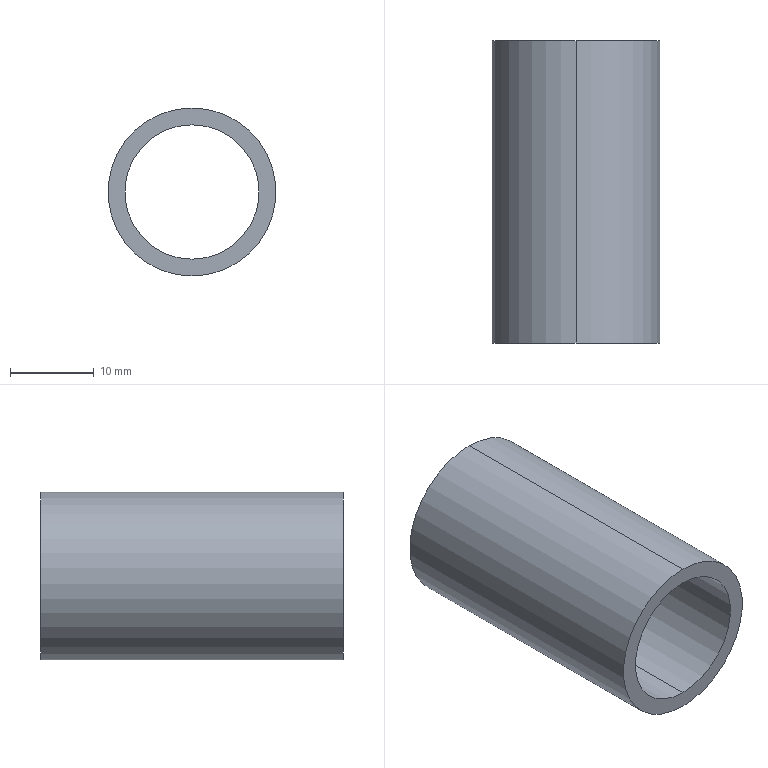Part | SolidWorks | features Extrusion 1 | 1 solid | 6 faces | box 20 x 36 x 20 mm | volume 4072 mm3 | cylinder 4 | plane 2 | commonest cylinder face diameters 16 x2 20 x2
STEP:
#1=CARTESIAN_POINT('',(0.,36.,-8.));
#2=VERTEX_POINT('',#1);
#3=CARTESIAN_POINT('',(0.,36.,8.));
#4=VERTEX_POINT('',#3);
#5=CARTESIAN_POINT('',(0.,36.,0.));
#6=DIRECTION('',(0.,1.,0.));
#7=DIRECTION('',(0.,0.,1.));
#8=AXIS2_PLACEMENT_3D('',#5,#6,#7);
#9=CIRCLE('',#8,8.);
#10=EDGE_CURVE('',#2,#4,#9,.T.);
#11=ORIENTED_EDGE('',*,*,#10,.T.);
#12=CARTESIAN_POINT('',(0.,0.,8.));
#13=VERTEX_POINT('',#12);
#14=CARTESIAN_POINT('',(0.,36.,8.));
#15=DIRECTION('',(0.,-1.,0.));
#16=VECTOR('',#15,1000.);
#17=LINE('',#14,#16);
#18=EDGE_CURVE('',#4,#13,#17,.T.);
#19=ORIENTED_EDGE('',*,*,#18,.T.);
#20=CARTESIAN_POINT('',(0.,0.,-8.));
#21=VERTEX_POINT('',#20);
#22=CARTESIAN_POINT('',(0.,0.,0.));
#23=DIRECTION('',(0.,1.,0.));
#24=DIRECTION('',(0.,0.,1.));
#25=AXIS2_PLACEMENT_3D('',#22,#23,#24);
#26=CIRCLE('',#25,8.);
#27=EDGE_CURVE('',#21,#13,#26,.T.);
#28=ORIENTED_EDGE('',*,*,#27,.F.);
#29=CARTESIAN_POINT('',(0.,36.,-8.));
#30=DIRECTION('',(0.,-1.,0.));
#31=VECTOR('',#30,1000.);
#32=LINE('',#29,#31);
#33=EDGE_CURVE('',#2,#21,#32,.T.);
#34=ORIENTED_EDGE('',*,*,#33,.F.);
#35=EDGE_LOOP('',(#11,#19,#28,#34));
#36=FACE_OUTER_BOUND('',#35,.T.);
#37=CARTESIAN_POINT('',(0.,36.,0.));
#38=DIRECTION('',(0.,-1.,0.));
#39=DIRECTION('',(0.,0.,-1.));
#40=AXIS2_PLACEMENT_3D('',#37,#38,#39);
#41=CYLINDRICAL_SURFACE('',#40,8.);
#42=ADVANCED_FACE('',(#36),#41,.F.);
#43=CARTESIAN_POINT('',(0.,36.,10.));
#44=VERTEX_POINT('',#43);
#45=CARTESIAN_POINT('',(0.,36.,-10.));
#46=VERTEX_POINT('',#45);
#47=CARTESIAN_POINT('',(0.,36.,0.));
#48=DIRECTION('',(0.,1.,0.));
#49=DIRECTION('',(0.,0.,1.));
#50=AXIS2_PLACEMENT_3D('',#47,#48,#49);
#51=CIRCLE('',#50,10.);
#52=EDGE_CURVE('',#44,#46,#51,.T.);
#53=ORIENTED_EDGE('',*,*,#52,.F.);
#54=CARTESIAN_POINT('',(0.,0.,10.));
#55=VERTEX_POINT('',#54);
#56=CARTESIAN_POINT('',(0.,36.,10.));
#57=DIRECTION('',(0.,-1.,0.));
#58=VECTOR('',#57,1000.);
#59=LINE('',#56,#58);
#60=EDGE_CURVE('',#44,#55,#59,.T.);
#61=ORIENTED_EDGE('',*,*,#60,.T.);
#62=CARTESIAN_POINT('',(0.,0.,-10.));
#63=VERTEX_POINT('',#62);
#64=CARTESIAN_POINT('',(0.,0.,0.));
#65=DIRECTION('',(0.,1.,0.));
#66=DIRECTION('',(0.,0.,1.));
#67=AXIS2_PLACEMENT_3D('',#64,#65,#66);
#68=CIRCLE('',#67,10.);
#69=EDGE_CURVE('',#55,#63,#68,.T.);
#70=ORIENTED_EDGE('',*,*,#69,.T.);
#71=CARTESIAN_POINT('',(0.,36.,-10.));
#72=DIRECTION('',(0.,-1.,0.));
#73=VECTOR('',#72,1000.);
#74=LINE('',#71,#73);
#75=EDGE_CURVE('',#46,#63,#74,.T.);
#76=ORIENTED_EDGE('',*,*,#75,.F.);
#77=EDGE_LOOP('',(#53,#61,#70,#76));
#78=FACE_OUTER_BOUND('',#77,.T.);
#79=CARTESIAN_POINT('',(0.,36.,0.));
#80=DIRECTION('',(0.,-1.,0.));
#81=DIRECTION('',(0.,0.,-1.));
#82=AXIS2_PLACEMENT_3D('',#79,#80,#81);
#83=CYLINDRICAL_SURFACE('',#82,10.);
#84=ADVANCED_FACE('',(#78),#83,.T.);
#85=CARTESIAN_POINT('',(0.,36.,0.));
#86=DIRECTION('',(0.,1.,0.));
#87=DIRECTION('',(0.,0.,1.));
#88=AXIS2_PLACEMENT_3D('',#85,#86,#87);
#89=CIRCLE('',#88,10.);
#90=EDGE_CURVE('',#46,#44,#89,.T.);
#91=ORIENTED_EDGE('',*,*,#90,.T.);
#92=ORIENTED_EDGE('',*,*,#52,.T.);
#93=EDGE_LOOP('',(#91,#92));
#94=FACE_OUTER_BOUND('',#93,.T.);
#95=ORIENTED_EDGE('',*,*,#10,.F.);
#96=CARTESIAN_POINT('',(0.,36.,0.));
#97=DIRECTION('',(0.,1.,0.));
#98=DIRECTION('',(0.,0.,1.));
#99=AXIS2_PLACEMENT_3D('',#96,#97,#98);
#100=CIRCLE('',#99,8.);
#101=EDGE_CURVE('',#4,#2,#100,.T.);
#102=ORIENTED_EDGE('',*,*,#101,.F.);
#103=EDGE_LOOP('',(#95,#102));
#104=FACE_BOUND('',#103,.T.);
#105=CARTESIAN_POINT('',(0.,36.,0.));
#106=DIRECTION('',(0.,1.,0.));
#107=DIRECTION('',(0.,0.,1.));
#108=AXIS2_PLACEMENT_3D('',#105,#106,#107);
#109=PLANE('',#108);
#110=ADVANCED_FACE('',(#94,#104),#109,.T.);
#111=CARTESIAN_POINT('',(0.,0.,0.));
#112=DIRECTION('',(0.,1.,0.));
#113=DIRECTION('',(0.,0.,1.));
#114=AXIS2_PLACEMENT_3D('',#111,#112,#113);
#115=CIRCLE('',#114,10.);
#116=EDGE_CURVE('',#63,#55,#115,.T.);
#117=ORIENTED_EDGE('',*,*,#116,.F.);
#118=ORIENTED_EDGE('',*,*,#69,.F.);
#119=EDGE_LOOP('',(#117,#118));
#120=FACE_OUTER_BOUND('',#119,.T.);
#121=ORIENTED_EDGE('',*,*,#27,.T.);
#122=CARTESIAN_POINT('',(0.,0.,0.));
#123=DIRECTION('',(0.,1.,0.));
#124=DIRECTION('',(0.,0.,1.));
#125=AXIS2_PLACEMENT_3D('',#122,#123,#124);
#126=CIRCLE('',#125,8.);
#127=EDGE_CURVE('',#13,#21,#126,.T.);
#128=ORIENTED_EDGE('',*,*,#127,.T.);
#129=EDGE_LOOP('',(#121,#128));
#130=FACE_BOUND('',#129,.T.);
#131=CARTESIAN_POINT('',(0.,0.,0.));
#132=DIRECTION('',(0.,1.,0.));
#133=DIRECTION('',(0.,0.,1.));
#134=AXIS2_PLACEMENT_3D('',#131,#132,#133);
#135=PLANE('',#134);
#136=ADVANCED_FACE('',(#120,#130),#135,.F.);
#137=ORIENTED_EDGE('',*,*,#60,.F.);
#138=ORIENTED_EDGE('',*,*,#90,.F.);
#139=ORIENTED_EDGE('',*,*,#75,.T.);
#140=ORIENTED_EDGE('',*,*,#116,.T.);
#141=EDGE_LOOP('',(#137,#138,#139,#140));
#142=FACE_OUTER_BOUND('',#141,.T.);
#143=CARTESIAN_POINT('',(0.,36.,0.));
#144=DIRECTION('',(0.,-1.,0.));
#145=DIRECTION('',(0.,0.,-1.));
#146=AXIS2_PLACEMENT_3D('',#143,#144,#145);
#147=CYLINDRICAL_SURFACE('',#146,10.);
#148=ADVANCED_FACE('',(#142),#147,.T.);
#149=ORIENTED_EDGE('',*,*,#18,.F.);
#150=ORIENTED_EDGE('',*,*,#101,.T.);
#151=ORIENTED_EDGE('',*,*,#33,.T.);
#152=ORIENTED_EDGE('',*,*,#127,.F.);
#153=EDGE_LOOP('',(#149,#150,#151,#152));
#154=FACE_OUTER_BOUND('',#153,.T.);
#155=CARTESIAN_POINT('',(0.,36.,0.));
#156=DIRECTION('',(0.,-1.,0.));
#157=DIRECTION('',(0.,0.,-1.));
#158=AXIS2_PLACEMENT_3D('',#155,#156,#157);
#159=CYLINDRICAL_SURFACE('',#158,8.);
#160=ADVANCED_FACE('',(#154),#159,.F.);
#161=CLOSED_SHELL('',(#42,#84,#110,#136,#148,#160));
#162=MANIFOLD_SOLID_BREP('',#161);
#163=CARTESIAN_POINT('',(0.,0.,0.));
#164=DIRECTION('',(0.,0.,1.));
#165=DIRECTION('',(1.,0.,0.));
#166=AXIS2_PLACEMENT_3D('',#163,#164,#165);
#167=(LENGTH_UNIT()NAMED_UNIT(*)SI_UNIT(.MILLI.,.METRE.));
#168=UNCERTAINTY_MEASURE_WITH_UNIT(LENGTH_MEASURE(0.00001),#167,'','');
#169=(NAMED_UNIT(*)PLANE_ANGLE_UNIT()SI_UNIT($,.RADIAN.));
#170=(NAMED_UNIT(*)SI_UNIT($,.STERADIAN.)SOLID_ANGLE_UNIT());
#171=(GEOMETRIC_REPRESENTATION_CONTEXT(3)GLOBAL_UNCERTAINTY_ASSIGNED_CONTEXT((#168))GLOBAL_UNIT_ASSIGNED_CONTEXT((#167,#169,#170))REPRESENTATION_CONTEXT('',''));
#172=ADVANCED_BREP_SHAPE_REPRESENTATION('',(#162,#166),#171);